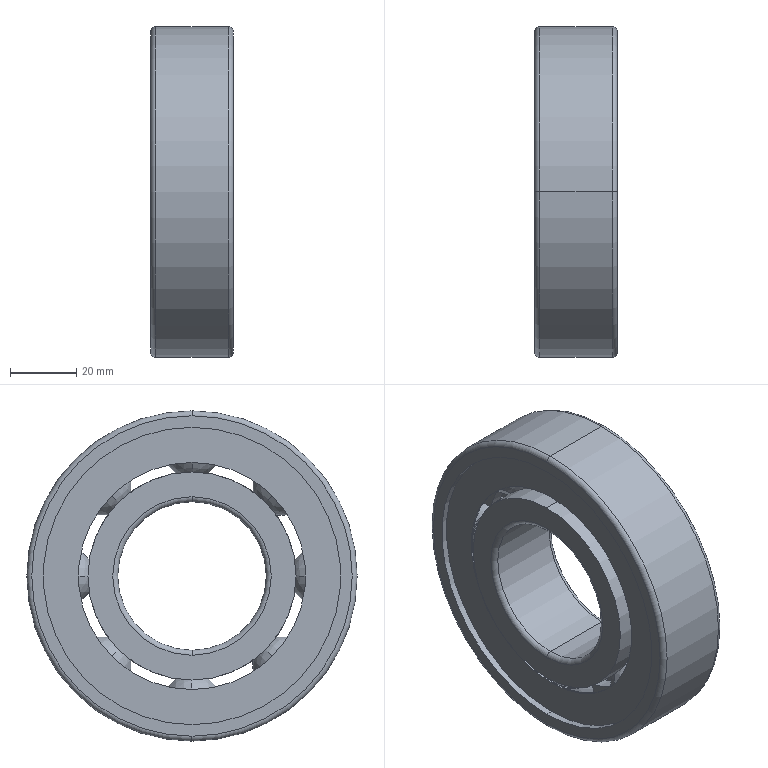Part | SolidWorks | features Revolution 6, CirPattern 2, RevCut 2, MirrorPattern 1 | 1 solid | 144 faces | box 25 x 100 x 100 mm | volume 96597 mm3 | sphere 64 | torus 32 | cylinder 24 | plane 24 | commonest cylinder face diameters 90 x8 63 x4 68.762 x4 45 x2 71.698 x2 81.302 x2